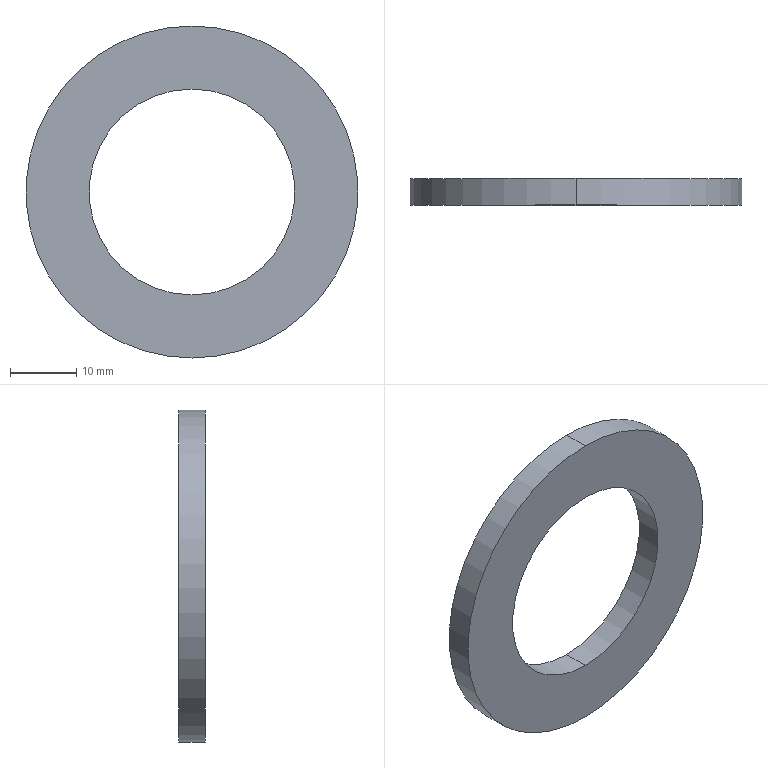Part | SolidWorks | features MirrorStock 1 | 1 solid | 6 faces | box 50 x 4 x 50 mm | volume 4835 mm3 | cylinder 4 | plane 2 | commonest cylinder face diameters 31 x2 50 x2
STEP:
#1=CARTESIAN_POINT('',(0.,2.,-15.5));
#2=VERTEX_POINT('',#1);
#3=CARTESIAN_POINT('',(0.,2.,15.5));
#4=VERTEX_POINT('',#3);
#5=CARTESIAN_POINT('',(0.,2.,0.));
#6=DIRECTION('',(0.,-1.,0.));
#7=DIRECTION('',(0.,0.,-1.));
#8=AXIS2_PLACEMENT_3D('',#5,#6,#7);
#9=CIRCLE('',#8,15.5);
#10=EDGE_CURVE('',#2,#4,#9,.T.);
#11=ORIENTED_EDGE('',*,*,#10,.F.);
#12=CARTESIAN_POINT('',(0.,-2.,-15.5));
#13=VERTEX_POINT('',#12);
#14=CARTESIAN_POINT('',(0.,2.,-15.5));
#15=DIRECTION('',(0.,-1.,0.));
#16=VECTOR('',#15,1000.);
#17=LINE('',#14,#16);
#18=EDGE_CURVE('',#2,#13,#17,.T.);
#19=ORIENTED_EDGE('',*,*,#18,.T.);
#20=CARTESIAN_POINT('',(0.,-2.,15.5));
#21=VERTEX_POINT('',#20);
#22=CARTESIAN_POINT('',(0.,-2.,0.));
#23=DIRECTION('',(0.,-1.,0.));
#24=DIRECTION('',(0.,0.,-1.));
#25=AXIS2_PLACEMENT_3D('',#22,#23,#24);
#26=CIRCLE('',#25,15.5);
#27=EDGE_CURVE('',#13,#21,#26,.T.);
#28=ORIENTED_EDGE('',*,*,#27,.T.);
#29=CARTESIAN_POINT('',(0.,2.,15.5));
#30=DIRECTION('',(0.,-1.,0.));
#31=VECTOR('',#30,1000.);
#32=LINE('',#29,#31);
#33=EDGE_CURVE('',#4,#21,#32,.T.);
#34=ORIENTED_EDGE('',*,*,#33,.F.);
#35=EDGE_LOOP('',(#11,#19,#28,#34));
#36=FACE_OUTER_BOUND('',#35,.T.);
#37=CARTESIAN_POINT('',(0.,2.,0.));
#38=DIRECTION('',(0.,-1.,0.));
#39=DIRECTION('',(0.,0.,1.));
#40=AXIS2_PLACEMENT_3D('',#37,#38,#39);
#41=CYLINDRICAL_SURFACE('',#40,15.5);
#42=ADVANCED_FACE('',(#36),#41,.F.);
#43=CARTESIAN_POINT('',(0.,2.,25.));
#44=VERTEX_POINT('',#43);
#45=CARTESIAN_POINT('',(0.,2.,-25.));
#46=VERTEX_POINT('',#45);
#47=CARTESIAN_POINT('',(0.,2.,0.));
#48=DIRECTION('',(0.,-1.,0.));
#49=DIRECTION('',(0.,0.,-1.));
#50=AXIS2_PLACEMENT_3D('',#47,#48,#49);
#51=CIRCLE('',#50,25.);
#52=EDGE_CURVE('',#44,#46,#51,.T.);
#53=ORIENTED_EDGE('',*,*,#52,.T.);
#54=CARTESIAN_POINT('',(0.,-2.,-25.));
#55=VERTEX_POINT('',#54);
#56=CARTESIAN_POINT('',(0.,2.,-25.));
#57=DIRECTION('',(0.,-1.,0.));
#58=VECTOR('',#57,1000.);
#59=LINE('',#56,#58);
#60=EDGE_CURVE('',#46,#55,#59,.T.);
#61=ORIENTED_EDGE('',*,*,#60,.T.);
#62=CARTESIAN_POINT('',(0.,-2.,25.));
#63=VERTEX_POINT('',#62);
#64=CARTESIAN_POINT('',(0.,-2.,0.));
#65=DIRECTION('',(0.,-1.,0.));
#66=DIRECTION('',(0.,0.,-1.));
#67=AXIS2_PLACEMENT_3D('',#64,#65,#66);
#68=CIRCLE('',#67,25.);
#69=EDGE_CURVE('',#63,#55,#68,.T.);
#70=ORIENTED_EDGE('',*,*,#69,.F.);
#71=CARTESIAN_POINT('',(0.,2.,25.));
#72=DIRECTION('',(0.,-1.,0.));
#73=VECTOR('',#72,1000.);
#74=LINE('',#71,#73);
#75=EDGE_CURVE('',#44,#63,#74,.T.);
#76=ORIENTED_EDGE('',*,*,#75,.F.);
#77=EDGE_LOOP('',(#53,#61,#70,#76));
#78=FACE_OUTER_BOUND('',#77,.T.);
#79=CARTESIAN_POINT('',(0.,2.,0.));
#80=DIRECTION('',(0.,-1.,0.));
#81=DIRECTION('',(0.,0.,1.));
#82=AXIS2_PLACEMENT_3D('',#79,#80,#81);
#83=CYLINDRICAL_SURFACE('',#82,25.);
#84=ADVANCED_FACE('',(#78),#83,.T.);
#85=ORIENTED_EDGE('',*,*,#52,.F.);
#86=CARTESIAN_POINT('',(0.,2.,0.));
#87=DIRECTION('',(0.,-1.,0.));
#88=DIRECTION('',(0.,0.,-1.));
#89=AXIS2_PLACEMENT_3D('',#86,#87,#88);
#90=CIRCLE('',#89,25.);
#91=EDGE_CURVE('',#46,#44,#90,.T.);
#92=ORIENTED_EDGE('',*,*,#91,.F.);
#93=EDGE_LOOP('',(#85,#92));
#94=FACE_OUTER_BOUND('',#93,.T.);
#95=CARTESIAN_POINT('',(0.,2.,0.));
#96=DIRECTION('',(0.,-1.,0.));
#97=DIRECTION('',(0.,0.,-1.));
#98=AXIS2_PLACEMENT_3D('',#95,#96,#97);
#99=CIRCLE('',#98,15.5);
#100=EDGE_CURVE('',#4,#2,#99,.T.);
#101=ORIENTED_EDGE('',*,*,#100,.T.);
#102=ORIENTED_EDGE('',*,*,#10,.T.);
#103=EDGE_LOOP('',(#101,#102));
#104=FACE_BOUND('',#103,.T.);
#105=CARTESIAN_POINT('',(0.,2.,0.));
#106=DIRECTION('',(0.,1.,0.));
#107=DIRECTION('',(0.,0.,-1.));
#108=AXIS2_PLACEMENT_3D('',#105,#106,#107);
#109=PLANE('',#108);
#110=ADVANCED_FACE('',(#94,#104),#109,.T.);
#111=ORIENTED_EDGE('',*,*,#69,.T.);
#112=CARTESIAN_POINT('',(0.,-2.,0.));
#113=DIRECTION('',(0.,-1.,0.));
#114=DIRECTION('',(0.,0.,-1.));
#115=AXIS2_PLACEMENT_3D('',#112,#113,#114);
#116=CIRCLE('',#115,25.);
#117=EDGE_CURVE('',#55,#63,#116,.T.);
#118=ORIENTED_EDGE('',*,*,#117,.T.);
#119=EDGE_LOOP('',(#111,#118));
#120=FACE_OUTER_BOUND('',#119,.T.);
#121=CARTESIAN_POINT('',(0.,-2.,0.));
#122=DIRECTION('',(0.,-1.,0.));
#123=DIRECTION('',(0.,0.,-1.));
#124=AXIS2_PLACEMENT_3D('',#121,#122,#123);
#125=CIRCLE('',#124,15.5);
#126=EDGE_CURVE('',#21,#13,#125,.T.);
#127=ORIENTED_EDGE('',*,*,#126,.F.);
#128=ORIENTED_EDGE('',*,*,#27,.F.);
#129=EDGE_LOOP('',(#127,#128));
#130=FACE_BOUND('',#129,.T.);
#131=CARTESIAN_POINT('',(0.,-2.,0.));
#132=DIRECTION('',(0.,1.,0.));
#133=DIRECTION('',(0.,0.,-1.));
#134=AXIS2_PLACEMENT_3D('',#131,#132,#133);
#135=PLANE('',#134);
#136=ADVANCED_FACE('',(#120,#130),#135,.F.);
#137=ORIENTED_EDGE('',*,*,#60,.F.);
#138=ORIENTED_EDGE('',*,*,#91,.T.);
#139=ORIENTED_EDGE('',*,*,#75,.T.);
#140=ORIENTED_EDGE('',*,*,#117,.F.);
#141=EDGE_LOOP('',(#137,#138,#139,#140));
#142=FACE_OUTER_BOUND('',#141,.T.);
#143=CARTESIAN_POINT('',(0.,2.,0.));
#144=DIRECTION('',(0.,-1.,0.));
#145=DIRECTION('',(0.,0.,1.));
#146=AXIS2_PLACEMENT_3D('',#143,#144,#145);
#147=CYLINDRICAL_SURFACE('',#146,25.);
#148=ADVANCED_FACE('',(#142),#147,.T.);
#149=ORIENTED_EDGE('',*,*,#18,.F.);
#150=ORIENTED_EDGE('',*,*,#100,.F.);
#151=ORIENTED_EDGE('',*,*,#33,.T.);
#152=ORIENTED_EDGE('',*,*,#126,.T.);
#153=EDGE_LOOP('',(#149,#150,#151,#152));
#154=FACE_OUTER_BOUND('',#153,.T.);
#155=CARTESIAN_POINT('',(0.,2.,0.));
#156=DIRECTION('',(0.,-1.,0.));
#157=DIRECTION('',(0.,0.,1.));
#158=AXIS2_PLACEMENT_3D('',#155,#156,#157);
#159=CYLINDRICAL_SURFACE('',#158,15.5);
#160=ADVANCED_FACE('',(#154),#159,.F.);
#161=CLOSED_SHELL('',(#42,#84,#110,#136,#148,#160));
#162=MANIFOLD_SOLID_BREP('',#161);
#163=CARTESIAN_POINT('',(0.,0.,0.));
#164=DIRECTION('',(0.,0.,1.));
#165=DIRECTION('',(1.,0.,0.));
#166=AXIS2_PLACEMENT_3D('',#163,#164,#165);
#167=(LENGTH_UNIT()NAMED_UNIT(*)SI_UNIT(.MILLI.,.METRE.));
#168=UNCERTAINTY_MEASURE_WITH_UNIT(LENGTH_MEASURE(0.00001),#167,'','');
#169=(NAMED_UNIT(*)PLANE_ANGLE_UNIT()SI_UNIT($,.RADIAN.));
#170=(NAMED_UNIT(*)SI_UNIT($,.STERADIAN.)SOLID_ANGLE_UNIT());
#171=(GEOMETRIC_REPRESENTATION_CONTEXT(3)GLOBAL_UNCERTAINTY_ASSIGNED_CONTEXT((#168))GLOBAL_UNIT_ASSIGNED_CONTEXT((#167,#169,#170))REPRESENTATION_CONTEXT('',''));
#172=ADVANCED_BREP_SHAPE_REPRESENTATION('',(#162,#166),#171);